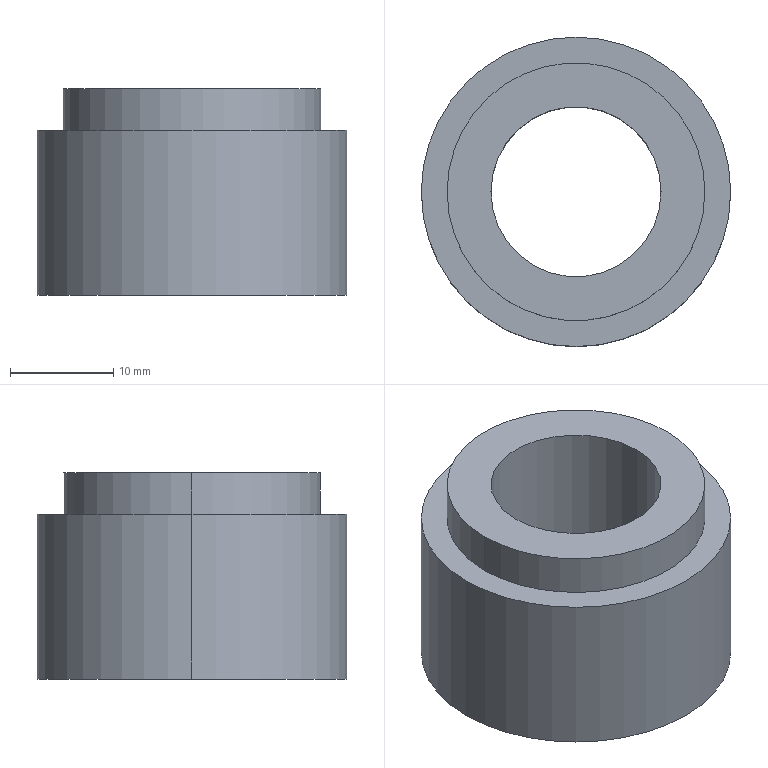Part | SolidWorks | features Chamfer 1, HoleWzd 1, Revolution 1 | 1 solid | 11 faces | box 30 x 30 x 20 mm | volume 8982 mm3 | cylinder 6 | plane 3 | cone 2 | commonest cylinder face diameters 16.5 x2 25 x2 30 x2
STEP:
#1=CARTESIAN_POINT('',(8.25,0.,-19.25));
#2=VERTEX_POINT('',#1);
#3=CARTESIAN_POINT('',(-8.25,0.,-19.25));
#4=VERTEX_POINT('',#3);
#5=CARTESIAN_POINT('',(0.,0.,-19.25));
#6=DIRECTION('',(0.,0.,-1.));
#7=DIRECTION('',(-1.,0.,0.));
#8=AXIS2_PLACEMENT_3D('',#5,#6,#7);
#9=CIRCLE('',#8,8.25);
#10=EDGE_CURVE('',#2,#4,#9,.T.);
#11=ORIENTED_EDGE('',*,*,#10,.F.);
#12=CARTESIAN_POINT('',(9.,0.,-20.));
#13=VERTEX_POINT('',#12);
#14=CARTESIAN_POINT('',(8.25,0.,-19.25));
#15=DIRECTION('',(0.7071,0.,-0.7071));
#16=VECTOR('',#15,1000.);
#17=LINE('',#14,#16);
#18=EDGE_CURVE('',#2,#13,#17,.T.);
#19=ORIENTED_EDGE('',*,*,#18,.T.);
#20=CARTESIAN_POINT('',(-9.,0.,-20.));
#21=VERTEX_POINT('',#20);
#22=CARTESIAN_POINT('',(0.,0.,-20.));
#23=DIRECTION('',(0.,0.,1.));
#24=DIRECTION('',(-1.,0.,0.));
#25=AXIS2_PLACEMENT_3D('',#22,#23,#24);
#26=CIRCLE('',#25,9.);
#27=EDGE_CURVE('',#21,#13,#26,.T.);
#28=ORIENTED_EDGE('',*,*,#27,.F.);
#29=CARTESIAN_POINT('',(-8.25,0.,-19.25));
#30=DIRECTION('',(-0.7071,0.,-0.7071));
#31=VECTOR('',#30,1000.);
#32=LINE('',#29,#31);
#33=EDGE_CURVE('',#4,#21,#32,.T.);
#34=ORIENTED_EDGE('',*,*,#33,.F.);
#35=EDGE_LOOP('',(#11,#19,#28,#34));
#36=FACE_OUTER_BOUND('',#35,.T.);
#37=CARTESIAN_POINT('',(0.,0.,-19.25));
#38=DIRECTION('',(0.,0.,-1.));
#39=DIRECTION('',(-1.,0.,0.));
#40=AXIS2_PLACEMENT_3D('',#37,#38,#39);
#41=CONICAL_SURFACE('',#40,8.25,0.7854);
#42=ADVANCED_FACE('',(#36),#41,.F.);
#43=CARTESIAN_POINT('',(-8.25,0.,0.));
#44=VERTEX_POINT('',#43);
#45=CARTESIAN_POINT('',(8.25,0.,0.));
#46=VERTEX_POINT('',#45);
#47=CARTESIAN_POINT('',(0.,0.,0.));
#48=DIRECTION('',(0.,0.,1.));
#49=DIRECTION('',(1.,0.,0.));
#50=AXIS2_PLACEMENT_3D('',#47,#48,#49);
#51=CIRCLE('',#50,8.25);
#52=EDGE_CURVE('',#44,#46,#51,.T.);
#53=ORIENTED_EDGE('',*,*,#52,.T.);
#54=CARTESIAN_POINT('',(8.25,0.,-20.));
#55=DIRECTION('',(0.,0.,-1.));
#56=VECTOR('',#55,1000.);
#57=LINE('',#54,#56);
#58=EDGE_CURVE('',#46,#2,#57,.T.);
#59=ORIENTED_EDGE('',*,*,#58,.T.);
#60=ORIENTED_EDGE('',*,*,#10,.T.);
#61=CARTESIAN_POINT('',(-8.25,0.,-20.));
#62=DIRECTION('',(0.,0.,-1.));
#63=VECTOR('',#62,1000.);
#64=LINE('',#61,#63);
#65=EDGE_CURVE('',#44,#4,#64,.T.);
#66=ORIENTED_EDGE('',*,*,#65,.F.);
#67=EDGE_LOOP('',(#53,#59,#60,#66));
#68=FACE_OUTER_BOUND('',#67,.T.);
#69=CARTESIAN_POINT('',(0.,0.,-20.));
#70=DIRECTION('',(0.,0.,-1.));
#71=DIRECTION('',(-1.,0.,0.));
#72=AXIS2_PLACEMENT_3D('',#69,#70,#71);
#73=CYLINDRICAL_SURFACE('',#72,8.25);
#74=ADVANCED_FACE('',(#68),#73,.F.);
#75=CARTESIAN_POINT('',(15.,0.,-20.));
#76=VERTEX_POINT('',#75);
#77=CARTESIAN_POINT('',(-15.,0.,-20.));
#78=VERTEX_POINT('',#77);
#79=CARTESIAN_POINT('',(0.,0.,-20.));
#80=DIRECTION('',(0.,0.,1.));
#81=DIRECTION('',(1.,0.,0.));
#82=AXIS2_PLACEMENT_3D('',#79,#80,#81);
#83=CIRCLE('',#82,15.);
#84=EDGE_CURVE('',#76,#78,#83,.T.);
#85=ORIENTED_EDGE('',*,*,#84,.T.);
#86=CARTESIAN_POINT('',(-15.,0.,-4.));
#87=VERTEX_POINT('',#86);
#88=CARTESIAN_POINT('',(-15.,0.,0.));
#89=DIRECTION('',(0.,0.,1.));
#90=VECTOR('',#89,1000.);
#91=LINE('',#88,#90);
#92=EDGE_CURVE('',#78,#87,#91,.T.);
#93=ORIENTED_EDGE('',*,*,#92,.T.);
#94=CARTESIAN_POINT('',(15.,0.,-4.));
#95=VERTEX_POINT('',#94);
#96=CARTESIAN_POINT('',(0.,0.,-4.));
#97=DIRECTION('',(0.,0.,1.));
#98=DIRECTION('',(1.,0.,0.));
#99=AXIS2_PLACEMENT_3D('',#96,#97,#98);
#100=CIRCLE('',#99,15.);
#101=EDGE_CURVE('',#95,#87,#100,.T.);
#102=ORIENTED_EDGE('',*,*,#101,.F.);
#103=CARTESIAN_POINT('',(15.,0.,0.));
#104=DIRECTION('',(0.,0.,1.));
#105=VECTOR('',#104,1000.);
#106=LINE('',#103,#105);
#107=EDGE_CURVE('',#76,#95,#106,.T.);
#108=ORIENTED_EDGE('',*,*,#107,.F.);
#109=EDGE_LOOP('',(#85,#93,#102,#108));
#110=FACE_OUTER_BOUND('',#109,.T.);
#111=CARTESIAN_POINT('',(0.,0.,0.));
#112=DIRECTION('',(0.,0.,1.));
#113=DIRECTION('',(1.,0.,0.));
#114=AXIS2_PLACEMENT_3D('',#111,#112,#113);
#115=CYLINDRICAL_SURFACE('',#114,15.);
#116=ADVANCED_FACE('',(#110),#115,.T.);
#117=CARTESIAN_POINT('',(12.5,0.,-4.));
#118=VERTEX_POINT('',#117);
#119=CARTESIAN_POINT('',(-12.5,0.,-4.));
#120=VERTEX_POINT('',#119);
#121=CARTESIAN_POINT('',(0.,0.,-4.));
#122=DIRECTION('',(0.,0.,1.));
#123=DIRECTION('',(1.,0.,0.));
#124=AXIS2_PLACEMENT_3D('',#121,#122,#123);
#125=CIRCLE('',#124,12.5);
#126=EDGE_CURVE('',#118,#120,#125,.T.);
#127=ORIENTED_EDGE('',*,*,#126,.T.);
#128=CARTESIAN_POINT('',(-12.5,0.,0.));
#129=VERTEX_POINT('',#128);
#130=CARTESIAN_POINT('',(-12.5,0.,0.));
#131=DIRECTION('',(0.,0.,1.));
#132=VECTOR('',#131,1000.);
#133=LINE('',#130,#132);
#134=EDGE_CURVE('',#120,#129,#133,.T.);
#135=ORIENTED_EDGE('',*,*,#134,.T.);
#136=CARTESIAN_POINT('',(12.5,0.,0.));
#137=VERTEX_POINT('',#136);
#138=CARTESIAN_POINT('',(0.,0.,0.));
#139=DIRECTION('',(0.,0.,1.));
#140=DIRECTION('',(1.,0.,0.));
#141=AXIS2_PLACEMENT_3D('',#138,#139,#140);
#142=CIRCLE('',#141,12.5);
#143=EDGE_CURVE('',#137,#129,#142,.T.);
#144=ORIENTED_EDGE('',*,*,#143,.F.);
#145=CARTESIAN_POINT('',(12.5,0.,0.));
#146=DIRECTION('',(0.,0.,1.));
#147=VECTOR('',#146,1000.);
#148=LINE('',#145,#147);
#149=EDGE_CURVE('',#118,#137,#148,.T.);
#150=ORIENTED_EDGE('',*,*,#149,.F.);
#151=EDGE_LOOP('',(#127,#135,#144,#150));
#152=FACE_OUTER_BOUND('',#151,.T.);
#153=CARTESIAN_POINT('',(0.,0.,0.));
#154=DIRECTION('',(0.,0.,1.));
#155=DIRECTION('',(1.,0.,0.));
#156=AXIS2_PLACEMENT_3D('',#153,#154,#155);
#157=CYLINDRICAL_SURFACE('',#156,12.5);
#158=ADVANCED_FACE('',(#152),#157,.T.);
#159=ORIENTED_EDGE('',*,*,#52,.F.);
#160=CARTESIAN_POINT('',(0.,0.,0.));
#161=DIRECTION('',(0.,0.,1.));
#162=DIRECTION('',(1.,0.,0.));
#163=AXIS2_PLACEMENT_3D('',#160,#161,#162);
#164=CIRCLE('',#163,8.25);
#165=EDGE_CURVE('',#46,#44,#164,.T.);
#166=ORIENTED_EDGE('',*,*,#165,.F.);
#167=EDGE_LOOP('',(#159,#166));
#168=FACE_BOUND('',#167,.T.);
#169=ORIENTED_EDGE('',*,*,#143,.T.);
#170=CARTESIAN_POINT('',(0.,0.,0.));
#171=DIRECTION('',(0.,0.,1.));
#172=DIRECTION('',(1.,0.,0.));
#173=AXIS2_PLACEMENT_3D('',#170,#171,#172);
#174=CIRCLE('',#173,12.5);
#175=EDGE_CURVE('',#129,#137,#174,.T.);
#176=ORIENTED_EDGE('',*,*,#175,.T.);
#177=EDGE_LOOP('',(#169,#176));
#178=FACE_OUTER_BOUND('',#177,.T.);
#179=CARTESIAN_POINT('',(7.5,0.,0.));
#180=DIRECTION('',(0.,0.,1.));
#181=DIRECTION('',(1.,0.,0.));
#182=AXIS2_PLACEMENT_3D('',#179,#180,#181);
#183=PLANE('',#182);
#184=ADVANCED_FACE('',(#168,#178),#183,.T.);
#185=ORIENTED_EDGE('',*,*,#134,.F.);
#186=CARTESIAN_POINT('',(0.,0.,-4.));
#187=DIRECTION('',(0.,0.,1.));
#188=DIRECTION('',(1.,0.,0.));
#189=AXIS2_PLACEMENT_3D('',#186,#187,#188);
#190=CIRCLE('',#189,12.5);
#191=EDGE_CURVE('',#120,#118,#190,.T.);
#192=ORIENTED_EDGE('',*,*,#191,.T.);
#193=ORIENTED_EDGE('',*,*,#149,.T.);
#194=ORIENTED_EDGE('',*,*,#175,.F.);
#195=EDGE_LOOP('',(#185,#192,#193,#194));
#196=FACE_OUTER_BOUND('',#195,.T.);
#197=CARTESIAN_POINT('',(0.,0.,0.));
#198=DIRECTION('',(0.,0.,1.));
#199=DIRECTION('',(1.,0.,0.));
#200=AXIS2_PLACEMENT_3D('',#197,#198,#199);
#201=CYLINDRICAL_SURFACE('',#200,12.5);
#202=ADVANCED_FACE('',(#196),#201,.T.);
#203=ORIENTED_EDGE('',*,*,#101,.T.);
#204=CARTESIAN_POINT('',(0.,0.,-4.));
#205=DIRECTION('',(0.,0.,1.));
#206=DIRECTION('',(1.,0.,0.));
#207=AXIS2_PLACEMENT_3D('',#204,#205,#206);
#208=CIRCLE('',#207,15.);
#209=EDGE_CURVE('',#87,#95,#208,.T.);
#210=ORIENTED_EDGE('',*,*,#209,.T.);
#211=EDGE_LOOP('',(#203,#210));
#212=FACE_OUTER_BOUND('',#211,.T.);
#213=ORIENTED_EDGE('',*,*,#126,.F.);
#214=ORIENTED_EDGE('',*,*,#191,.F.);
#215=EDGE_LOOP('',(#213,#214));
#216=FACE_BOUND('',#215,.T.);
#217=CARTESIAN_POINT('',(12.5,0.,-4.));
#218=DIRECTION('',(0.,0.,1.));
#219=DIRECTION('',(1.,0.,0.));
#220=AXIS2_PLACEMENT_3D('',#217,#218,#219);
#221=PLANE('',#220);
#222=ADVANCED_FACE('',(#212,#216),#221,.T.);
#223=ORIENTED_EDGE('',*,*,#92,.F.);
#224=CARTESIAN_POINT('',(0.,0.,-20.));
#225=DIRECTION('',(0.,0.,1.));
#226=DIRECTION('',(1.,0.,0.));
#227=AXIS2_PLACEMENT_3D('',#224,#225,#226);
#228=CIRCLE('',#227,15.);
#229=EDGE_CURVE('',#78,#76,#228,.T.);
#230=ORIENTED_EDGE('',*,*,#229,.T.);
#231=ORIENTED_EDGE('',*,*,#107,.T.);
#232=ORIENTED_EDGE('',*,*,#209,.F.);
#233=EDGE_LOOP('',(#223,#230,#231,#232));
#234=FACE_OUTER_BOUND('',#233,.T.);
#235=CARTESIAN_POINT('',(0.,0.,0.));
#236=DIRECTION('',(0.,0.,1.));
#237=DIRECTION('',(1.,0.,0.));
#238=AXIS2_PLACEMENT_3D('',#235,#236,#237);
#239=CYLINDRICAL_SURFACE('',#238,15.);
#240=ADVANCED_FACE('',(#234),#239,.T.);
#241=ORIENTED_EDGE('',*,*,#27,.T.);
#242=CARTESIAN_POINT('',(0.,0.,-20.));
#243=DIRECTION('',(0.,0.,1.));
#244=DIRECTION('',(-1.,0.,0.));
#245=AXIS2_PLACEMENT_3D('',#242,#243,#244);
#246=CIRCLE('',#245,9.);
#247=EDGE_CURVE('',#13,#21,#246,.T.);
#248=ORIENTED_EDGE('',*,*,#247,.T.);
#249=EDGE_LOOP('',(#241,#248));
#250=FACE_BOUND('',#249,.T.);
#251=ORIENTED_EDGE('',*,*,#84,.F.);
#252=ORIENTED_EDGE('',*,*,#229,.F.);
#253=EDGE_LOOP('',(#251,#252));
#254=FACE_OUTER_BOUND('',#253,.T.);
#255=CARTESIAN_POINT('',(15.,0.,-20.));
#256=DIRECTION('',(0.,0.,-1.));
#257=DIRECTION('',(-1.,0.,0.));
#258=AXIS2_PLACEMENT_3D('',#255,#256,#257);
#259=PLANE('',#258);
#260=ADVANCED_FACE('',(#250,#254),#259,.T.);
#261=ORIENTED_EDGE('',*,*,#58,.F.);
#262=ORIENTED_EDGE('',*,*,#165,.T.);
#263=ORIENTED_EDGE('',*,*,#65,.T.);
#264=CARTESIAN_POINT('',(0.,0.,-19.25));
#265=DIRECTION('',(0.,0.,-1.));
#266=DIRECTION('',(-1.,0.,0.));
#267=AXIS2_PLACEMENT_3D('',#264,#265,#266);
#268=CIRCLE('',#267,8.25);
#269=EDGE_CURVE('',#4,#2,#268,.T.);
#270=ORIENTED_EDGE('',*,*,#269,.T.);
#271=EDGE_LOOP('',(#261,#262,#263,#270));
#272=FACE_OUTER_BOUND('',#271,.T.);
#273=CARTESIAN_POINT('',(0.,0.,-20.));
#274=DIRECTION('',(0.,0.,-1.));
#275=DIRECTION('',(-1.,0.,0.));
#276=AXIS2_PLACEMENT_3D('',#273,#274,#275);
#277=CYLINDRICAL_SURFACE('',#276,8.25);
#278=ADVANCED_FACE('',(#272),#277,.F.);
#279=ORIENTED_EDGE('',*,*,#18,.F.);
#280=ORIENTED_EDGE('',*,*,#269,.F.);
#281=ORIENTED_EDGE('',*,*,#33,.T.);
#282=ORIENTED_EDGE('',*,*,#247,.F.);
#283=EDGE_LOOP('',(#279,#280,#281,#282));
#284=FACE_OUTER_BOUND('',#283,.T.);
#285=CARTESIAN_POINT('',(0.,0.,-19.25));
#286=DIRECTION('',(0.,0.,-1.));
#287=DIRECTION('',(-1.,0.,0.));
#288=AXIS2_PLACEMENT_3D('',#285,#286,#287);
#289=CONICAL_SURFACE('',#288,8.25,0.7854);
#290=ADVANCED_FACE('',(#284),#289,.F.);
#291=CLOSED_SHELL('',(#42,#74,#116,#158,#184,#202,#222,#240,#260,#278,#290));
#292=MANIFOLD_SOLID_BREP('',#291);
#293=CARTESIAN_POINT('',(0.,0.,0.));
#294=DIRECTION('',(0.,0.,1.));
#295=DIRECTION('',(1.,0.,0.));
#296=AXIS2_PLACEMENT_3D('',#293,#294,#295);
#297=(LENGTH_UNIT()NAMED_UNIT(*)SI_UNIT(.MILLI.,.METRE.));
#298=UNCERTAINTY_MEASURE_WITH_UNIT(LENGTH_MEASURE(0.00001),#297,'','');
#299=(NAMED_UNIT(*)PLANE_ANGLE_UNIT()SI_UNIT($,.RADIAN.));
#300=(NAMED_UNIT(*)SI_UNIT($,.STERADIAN.)SOLID_ANGLE_UNIT());
#301=(GEOMETRIC_REPRESENTATION_CONTEXT(3)GLOBAL_UNCERTAINTY_ASSIGNED_CONTEXT((#298))GLOBAL_UNIT_ASSIGNED_CONTEXT((#297,#299,#300))REPRESENTATION_CONTEXT('',''));
#302=ADVANCED_BREP_SHAPE_REPRESENTATION('',(#292,#296),#301);